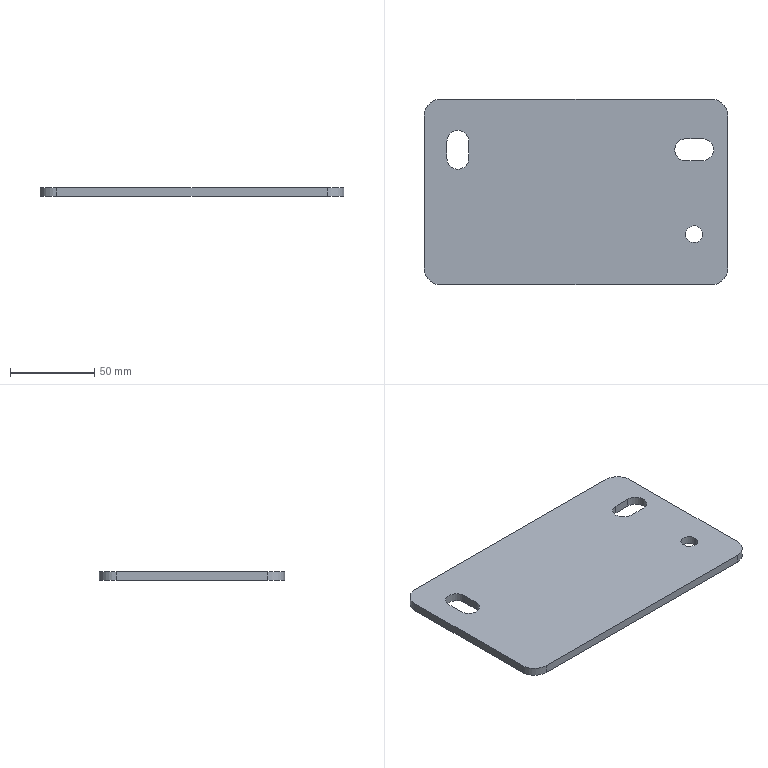Part | STEP file | IN-01-01-01-01 | 1 solid | 21 faces | box 180 x 110 x 5 mm | volume 95551 mm3 | cylinder 11 | plane 10 | commonest cylinder face diameters 13 x5 20 x4 10 x2